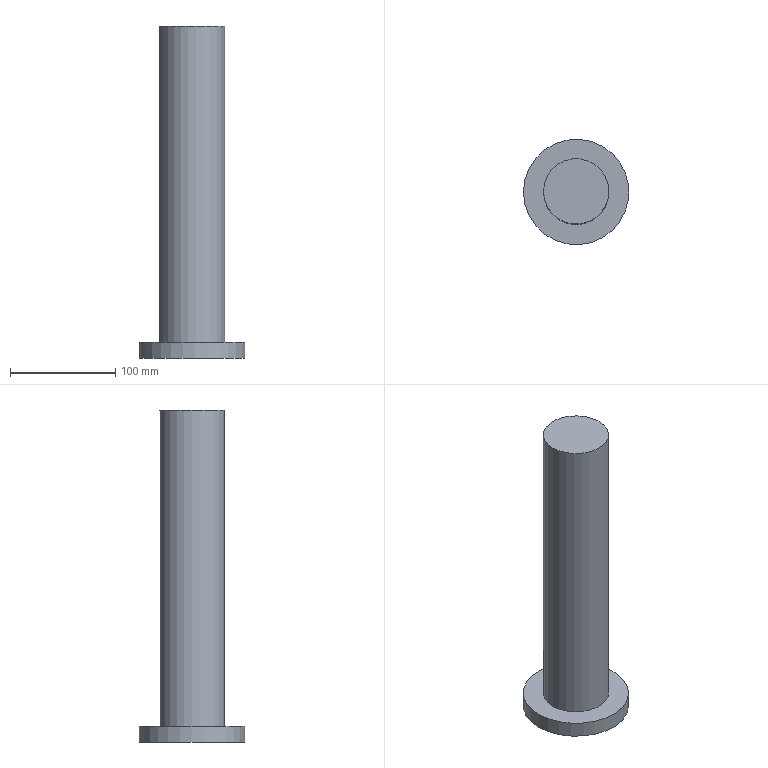Part | NX | features 推移杆柱销 2 | 1 solid | 5 faces | box 100 x 100 x 315 mm | volume 1023531 mm3 | plane 3 | cylinder 2 | commonest cylinder face diameters 62 x1 100 x1
STEP:
#1=CARTESIAN_POINT('',(31.,0.,300.));
#2=VERTEX_POINT('',#1);
#3=CARTESIAN_POINT('',(0.,0.,300.));
#4=DIRECTION('',(0.,0.,1.));
#5=DIRECTION('',(1.,0.,0.));
#6=AXIS2_PLACEMENT_3D('',#3,#4,#5);
#7=CIRCLE('',#6,31.);
#8=EDGE_CURVE('',#2,#2,#7,.T.);
#9=ORIENTED_EDGE('',*,*,#8,.F.);
#10=EDGE_LOOP('',(#9));
#11=FACE_BOUND('',#10,.T.);
#12=CARTESIAN_POINT('',(-31.,0.,0.));
#13=VERTEX_POINT('',#12);
#14=CARTESIAN_POINT('',(0.,0.,0.));
#15=DIRECTION('',(0.,0.,-1.));
#16=DIRECTION('',(-1.,0.,0.));
#17=AXIS2_PLACEMENT_3D('',#14,#15,#16);
#18=CIRCLE('',#17,31.);
#19=EDGE_CURVE('',#13,#13,#18,.T.);
#20=ORIENTED_EDGE('',*,*,#19,.F.);
#21=EDGE_LOOP('',(#20));
#22=FACE_BOUND('',#21,.T.);
#23=CARTESIAN_POINT('',(0.,0.,300.));
#24=DIRECTION('',(0.,0.,-1.));
#25=DIRECTION('',(-1.,0.,0.));
#26=AXIS2_PLACEMENT_3D('',#23,#24,#25);
#27=CYLINDRICAL_SURFACE('',#26,31.);
#28=ADVANCED_FACE('',(#11,#22),#27,.T.);
#29=ORIENTED_EDGE('',*,*,#8,.T.);
#30=EDGE_LOOP('',(#29));
#31=FACE_BOUND('',#30,.T.);
#32=CARTESIAN_POINT('',(0.,0.,300.));
#33=DIRECTION('',(0.,0.,1.));
#34=DIRECTION('',(1.,0.,0.));
#35=AXIS2_PLACEMENT_3D('',#32,#33,#34);
#36=PLANE('',#35);
#37=ADVANCED_FACE('',(#31),#36,.T.);
#38=CARTESIAN_POINT('',(-50.,0.,0.));
#39=VERTEX_POINT('',#38);
#40=CARTESIAN_POINT('',(0.,0.,0.));
#41=DIRECTION('',(0.,0.,-1.));
#42=DIRECTION('',(-1.,0.,0.));
#43=AXIS2_PLACEMENT_3D('',#40,#41,#42);
#44=CIRCLE('',#43,50.);
#45=EDGE_CURVE('',#39,#39,#44,.T.);
#46=ORIENTED_EDGE('',*,*,#45,.F.);
#47=EDGE_LOOP('',(#46));
#48=FACE_BOUND('',#47,.T.);
#49=ORIENTED_EDGE('',*,*,#19,.T.);
#50=EDGE_LOOP('',(#49));
#51=FACE_BOUND('',#50,.T.);
#52=CARTESIAN_POINT('',(0.,0.,0.));
#53=DIRECTION('',(0.,0.,-1.));
#54=DIRECTION('',(-1.,0.,0.));
#55=AXIS2_PLACEMENT_3D('',#52,#53,#54);
#56=PLANE('',#55);
#57=ADVANCED_FACE('',(#48,#51),#56,.F.);
#58=CARTESIAN_POINT('',(-50.,0.,-15.));
#59=VERTEX_POINT('',#58);
#60=CARTESIAN_POINT('',(0.,0.,-15.));
#61=DIRECTION('',(0.,0.,-1.));
#62=DIRECTION('',(-1.,0.,0.));
#63=AXIS2_PLACEMENT_3D('',#60,#61,#62);
#64=CIRCLE('',#63,50.);
#65=EDGE_CURVE('',#59,#59,#64,.T.);
#66=ORIENTED_EDGE('',*,*,#65,.F.);
#67=EDGE_LOOP('',(#66));
#68=FACE_BOUND('',#67,.T.);
#69=ORIENTED_EDGE('',*,*,#45,.T.);
#70=EDGE_LOOP('',(#69));
#71=FACE_BOUND('',#70,.T.);
#72=CARTESIAN_POINT('',(0.,0.,-15.));
#73=DIRECTION('',(0.,0.,1.));
#74=DIRECTION('',(1.,0.,0.));
#75=AXIS2_PLACEMENT_3D('',#72,#73,#74);
#76=CYLINDRICAL_SURFACE('',#75,50.);
#77=ADVANCED_FACE('',(#68,#71),#76,.T.);
#78=ORIENTED_EDGE('',*,*,#65,.T.);
#79=EDGE_LOOP('',(#78));
#80=FACE_BOUND('',#79,.T.);
#81=CARTESIAN_POINT('',(0.,0.,-15.));
#82=DIRECTION('',(0.,0.,-1.));
#83=DIRECTION('',(-1.,0.,0.));
#84=AXIS2_PLACEMENT_3D('',#81,#82,#83);
#85=PLANE('',#84);
#86=ADVANCED_FACE('',(#80),#85,.T.);
#87=CLOSED_SHELL('',(#28,#37,#57,#77,#86));
#88=MANIFOLD_SOLID_BREP('',#87);
#89=(LENGTH_UNIT()NAMED_UNIT(*)SI_UNIT(.MILLI.,.METRE.));
#90=UNCERTAINTY_MEASURE_WITH_UNIT(LENGTH_MEASURE(0.00001),#89,'','');
#91=(NAMED_UNIT(*)PLANE_ANGLE_UNIT()SI_UNIT($,.RADIAN.));
#92=(NAMED_UNIT(*)SI_UNIT($,.STERADIAN.)SOLID_ANGLE_UNIT());
#93=(GEOMETRIC_REPRESENTATION_CONTEXT(3)GLOBAL_UNCERTAINTY_ASSIGNED_CONTEXT((#90))GLOBAL_UNIT_ASSIGNED_CONTEXT((#89,#91,#92))REPRESENTATION_CONTEXT('',''));
#94=ADVANCED_BREP_SHAPE_REPRESENTATION('',(#88),#93);